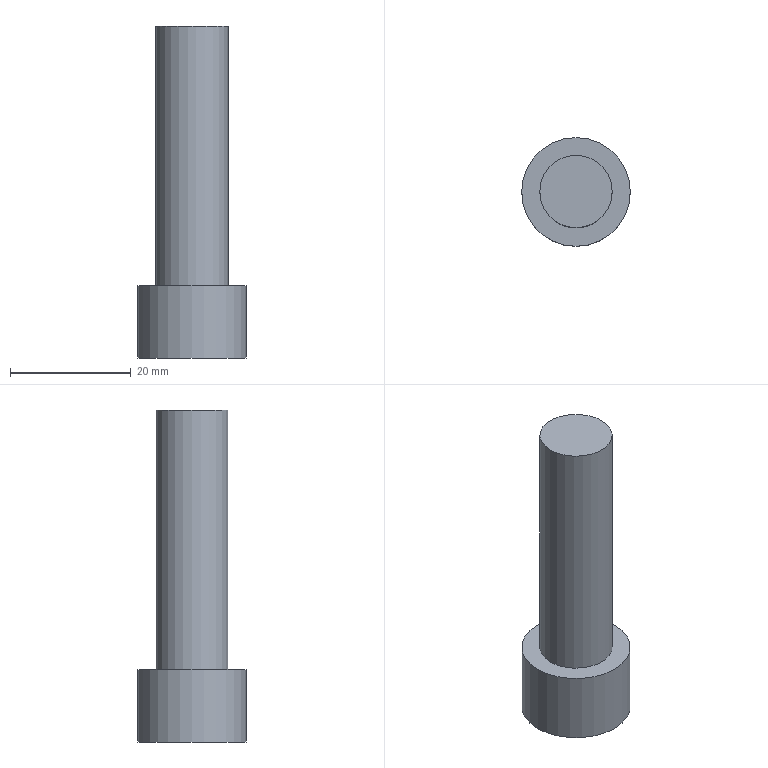Part | STEP file | 1_id610_xmt_txt | 1 solid | 18 faces | box 18 x 18 x 55 mm | volume 7362 mm3 | plane 15 | cylinder 2 | cone 1 | commonest cylinder face diameters 12 x1 18 x1
STEP:
#1=CARTESIAN_POINT('',(-111.,327.,-232.));
#2=VERTEX_POINT('',#1);
#3=CARTESIAN_POINT('',(-117.,327.,-232.));
#4=DIRECTION('',(0.,0.,-1.));
#5=DIRECTION('',(1.,0.,0.));
#6=AXIS2_PLACEMENT_3D('',#3,#4,#5);
#7=CIRCLE('',#6,6.);
#8=EDGE_CURVE('',#2,#2,#7,.T.);
#9=ORIENTED_EDGE('',*,*,#8,.F.);
#10=EDGE_LOOP('',(#9));
#11=FACE_BOUND('',#10,.T.);
#12=CARTESIAN_POINT('',(-111.,327.,-189.));
#13=VERTEX_POINT('',#12);
#14=CARTESIAN_POINT('',(-117.,327.,-189.));
#15=DIRECTION('',(0.,0.,1.));
#16=DIRECTION('',(1.,0.,0.));
#17=AXIS2_PLACEMENT_3D('',#14,#15,#16);
#18=CIRCLE('',#17,6.);
#19=EDGE_CURVE('',#13,#13,#18,.T.);
#20=ORIENTED_EDGE('',*,*,#19,.F.);
#21=EDGE_LOOP('',(#20));
#22=FACE_BOUND('',#21,.T.);
#23=CARTESIAN_POINT('',(-117.,327.,-212.));
#24=DIRECTION('',(0.,0.,1.));
#25=DIRECTION('',(-1.,0.,0.));
#26=AXIS2_PLACEMENT_3D('',#23,#24,#25);
#27=CYLINDRICAL_SURFACE('',#26,6.);
#28=ADVANCED_FACE('',(#11,#22),#27,.T.);
#29=CARTESIAN_POINT('',(-108.,327.,-244.));
#30=VERTEX_POINT('',#29);
#31=CARTESIAN_POINT('',(-117.,327.,-244.));
#32=DIRECTION('',(0.,0.,-1.));
#33=DIRECTION('',(1.,0.,0.));
#34=AXIS2_PLACEMENT_3D('',#31,#32,#33);
#35=CIRCLE('',#34,9.);
#36=EDGE_CURVE('',#30,#30,#35,.T.);
#37=ORIENTED_EDGE('',*,*,#36,.F.);
#38=EDGE_LOOP('',(#37));
#39=FACE_BOUND('',#38,.T.);
#40=CARTESIAN_POINT('',(-108.,327.,-232.));
#41=VERTEX_POINT('',#40);
#42=CARTESIAN_POINT('',(-117.,327.,-232.));
#43=DIRECTION('',(0.,0.,1.));
#44=DIRECTION('',(1.,0.,0.));
#45=AXIS2_PLACEMENT_3D('',#42,#43,#44);
#46=CIRCLE('',#45,9.);
#47=EDGE_CURVE('',#41,#41,#46,.T.);
#48=ORIENTED_EDGE('',*,*,#47,.F.);
#49=EDGE_LOOP('',(#48));
#50=FACE_BOUND('',#49,.T.);
#51=CARTESIAN_POINT('',(-117.,327.,-238.));
#52=DIRECTION('',(0.,0.,1.));
#53=DIRECTION('',(-1.,0.,0.));
#54=AXIS2_PLACEMENT_3D('',#51,#52,#53);
#55=CYLINDRICAL_SURFACE('',#54,9.);
#56=ADVANCED_FACE('',(#39,#50),#55,.T.);
#57=CARTESIAN_POINT('',(-117.,332.774,-238.));
#58=VERTEX_POINT('',#57);
#59=CARTESIAN_POINT('',(-112.,329.887,-238.));
#60=VERTEX_POINT('',#59);
#61=CARTESIAN_POINT('',(-117.,327.,-238.));
#62=DIRECTION('',(0.,0.,-1.));
#63=DIRECTION('',(1.,0.,0.));
#64=AXIS2_PLACEMENT_3D('',#61,#62,#63);
#65=CIRCLE('',#64,5.774);
#66=EDGE_CURVE('',#58,#60,#65,.T.);
#67=ORIENTED_EDGE('',*,*,#66,.T.);
#68=CARTESIAN_POINT('',(-112.,324.113,-238.));
#69=VERTEX_POINT('',#68);
#70=CARTESIAN_POINT('',(-117.,327.,-238.));
#71=DIRECTION('',(0.,0.,-1.));
#72=DIRECTION('',(1.,0.,0.));
#73=AXIS2_PLACEMENT_3D('',#70,#71,#72);
#74=CIRCLE('',#73,5.774);
#75=EDGE_CURVE('',#60,#69,#74,.T.);
#76=ORIENTED_EDGE('',*,*,#75,.T.);
#77=CARTESIAN_POINT('',(-117.,321.226,-238.));
#78=VERTEX_POINT('',#77);
#79=CARTESIAN_POINT('',(-117.,327.,-238.));
#80=DIRECTION('',(0.,0.,-1.));
#81=DIRECTION('',(1.,0.,0.));
#82=AXIS2_PLACEMENT_3D('',#79,#80,#81);
#83=CIRCLE('',#82,5.774);
#84=EDGE_CURVE('',#69,#78,#83,.T.);
#85=ORIENTED_EDGE('',*,*,#84,.T.);
#86=CARTESIAN_POINT('',(-122.,324.113,-238.));
#87=VERTEX_POINT('',#86);
#88=CARTESIAN_POINT('',(-117.,327.,-238.));
#89=DIRECTION('',(0.,0.,-1.));
#90=DIRECTION('',(1.,0.,0.));
#91=AXIS2_PLACEMENT_3D('',#88,#89,#90);
#92=CIRCLE('',#91,5.774);
#93=EDGE_CURVE('',#78,#87,#92,.T.);
#94=ORIENTED_EDGE('',*,*,#93,.T.);
#95=CARTESIAN_POINT('',(-122.,329.887,-238.));
#96=VERTEX_POINT('',#95);
#97=CARTESIAN_POINT('',(-117.,327.,-238.));
#98=DIRECTION('',(0.,0.,-1.));
#99=DIRECTION('',(1.,0.,0.));
#100=AXIS2_PLACEMENT_3D('',#97,#98,#99);
#101=CIRCLE('',#100,5.774);
#102=EDGE_CURVE('',#87,#96,#101,.T.);
#103=ORIENTED_EDGE('',*,*,#102,.T.);
#104=CARTESIAN_POINT('',(-117.,327.,-238.));
#105=DIRECTION('',(0.,0.,-1.));
#106=DIRECTION('',(1.,0.,0.));
#107=AXIS2_PLACEMENT_3D('',#104,#105,#106);
#108=CIRCLE('',#107,5.774);
#109=EDGE_CURVE('',#96,#58,#108,.T.);
#110=ORIENTED_EDGE('',*,*,#109,.T.);
#111=EDGE_LOOP('',(#67,#76,#85,#94,#103,#110));
#112=FACE_BOUND('',#111,.T.);
#113=CARTESIAN_POINT('',(-117.,327.,-237.));
#114=VERTEX_POINT('',#113);
#115=VERTEX_LOOP('',#114);
#116=FACE_BOUND('',#115,.T.);
#117=CARTESIAN_POINT('',(-117.,327.,-237.5));
#118=DIRECTION('',(0.,0.,-1.));
#119=DIRECTION('',(-1.,0.,0.));
#120=AXIS2_PLACEMENT_3D('',#117,#118,#119);
#121=CONICAL_SURFACE('',#120,2.887,80.174);
#122=ADVANCED_FACE('',(#112,#116),#121,.F.);
#123=CARTESIAN_POINT('',(-114.5,322.67,-238.));
#124=DIRECTION('',(0.866,0.5,0.));
#125=VECTOR('',#124,1.);
#126=LINE('',#123,#125);
#127=EDGE_CURVE('',#78,#69,#126,.T.);
#128=ORIENTED_EDGE('',*,*,#127,.F.);
#129=ORIENTED_EDGE('',*,*,#84,.F.);
#130=EDGE_LOOP('',(#128,#129));
#131=FACE_OUTER_BOUND('',#130,.T.);
#132=CARTESIAN_POINT('',(-117.,327.,-238.));
#133=DIRECTION('',(0.,0.,-1.));
#134=DIRECTION('',(1.,0.,0.));
#135=AXIS2_PLACEMENT_3D('',#132,#133,#134);
#136=PLANE('',#135);
#137=ADVANCED_FACE('',(#131),#136,.F.);
#138=CARTESIAN_POINT('',(-112.,327.,-238.));
#139=DIRECTION('',(0.,1.,0.));
#140=VECTOR('',#139,1.);
#141=LINE('',#138,#140);
#142=EDGE_CURVE('',#69,#60,#141,.T.);
#143=ORIENTED_EDGE('',*,*,#142,.F.);
#144=ORIENTED_EDGE('',*,*,#75,.F.);
#145=EDGE_LOOP('',(#143,#144));
#146=FACE_OUTER_BOUND('',#145,.T.);
#147=CARTESIAN_POINT('',(-117.,327.,-238.));
#148=DIRECTION('',(0.,0.,-1.));
#149=DIRECTION('',(1.,0.,0.));
#150=AXIS2_PLACEMENT_3D('',#147,#148,#149);
#151=PLANE('',#150);
#152=ADVANCED_FACE('',(#146),#151,.F.);
#153=CARTESIAN_POINT('',(-114.5,331.33,-238.));
#154=DIRECTION('',(-0.866,0.5,0.));
#155=VECTOR('',#154,1.);
#156=LINE('',#153,#155);
#157=EDGE_CURVE('',#60,#58,#156,.T.);
#158=ORIENTED_EDGE('',*,*,#157,.F.);
#159=ORIENTED_EDGE('',*,*,#66,.F.);
#160=EDGE_LOOP('',(#158,#159));
#161=FACE_OUTER_BOUND('',#160,.T.);
#162=CARTESIAN_POINT('',(-117.,327.,-238.));
#163=DIRECTION('',(0.,0.,-1.));
#164=DIRECTION('',(1.,0.,0.));
#165=AXIS2_PLACEMENT_3D('',#162,#163,#164);
#166=PLANE('',#165);
#167=ADVANCED_FACE('',(#161),#166,.F.);
#168=CARTESIAN_POINT('',(-119.5,331.33,-238.));
#169=DIRECTION('',(-0.866,-0.5,0.));
#170=VECTOR('',#169,1.);
#171=LINE('',#168,#170);
#172=EDGE_CURVE('',#58,#96,#171,.T.);
#173=ORIENTED_EDGE('',*,*,#172,.F.);
#174=ORIENTED_EDGE('',*,*,#109,.F.);
#175=EDGE_LOOP('',(#173,#174));
#176=FACE_OUTER_BOUND('',#175,.T.);
#177=CARTESIAN_POINT('',(-117.,327.,-238.));
#178=DIRECTION('',(0.,0.,-1.));
#179=DIRECTION('',(1.,0.,0.));
#180=AXIS2_PLACEMENT_3D('',#177,#178,#179);
#181=PLANE('',#180);
#182=ADVANCED_FACE('',(#176),#181,.F.);
#183=CARTESIAN_POINT('',(-122.,327.,-238.));
#184=DIRECTION('',(0.,-1.,0.));
#185=VECTOR('',#184,1.);
#186=LINE('',#183,#185);
#187=EDGE_CURVE('',#96,#87,#186,.T.);
#188=ORIENTED_EDGE('',*,*,#187,.F.);
#189=ORIENTED_EDGE('',*,*,#102,.F.);
#190=EDGE_LOOP('',(#188,#189));
#191=FACE_OUTER_BOUND('',#190,.T.);
#192=CARTESIAN_POINT('',(-117.,327.,-238.));
#193=DIRECTION('',(0.,0.,-1.));
#194=DIRECTION('',(1.,0.,0.));
#195=AXIS2_PLACEMENT_3D('',#192,#193,#194);
#196=PLANE('',#195);
#197=ADVANCED_FACE('',(#191),#196,.F.);
#198=CARTESIAN_POINT('',(-119.5,322.67,-238.));
#199=DIRECTION('',(0.866,-0.5,0.));
#200=VECTOR('',#199,1.);
#201=LINE('',#198,#200);
#202=EDGE_CURVE('',#87,#78,#201,.T.);
#203=ORIENTED_EDGE('',*,*,#202,.F.);
#204=ORIENTED_EDGE('',*,*,#93,.F.);
#205=EDGE_LOOP('',(#203,#204));
#206=FACE_OUTER_BOUND('',#205,.T.);
#207=CARTESIAN_POINT('',(-117.,327.,-238.));
#208=DIRECTION('',(0.,0.,-1.));
#209=DIRECTION('',(1.,0.,0.));
#210=AXIS2_PLACEMENT_3D('',#207,#208,#209);
#211=PLANE('',#210);
#212=ADVANCED_FACE('',(#206),#211,.F.);
#213=CARTESIAN_POINT('',(-117.,321.226,-244.));
#214=VERTEX_POINT('',#213);
#215=CARTESIAN_POINT('',(-117.,321.226,-241.));
#216=DIRECTION('',(0.,0.,-1.));
#217=VECTOR('',#216,1.);
#218=LINE('',#215,#217);
#219=EDGE_CURVE('',#78,#214,#218,.T.);
#220=ORIENTED_EDGE('',*,*,#219,.F.);
#221=ORIENTED_EDGE('',*,*,#127,.T.);
#222=CARTESIAN_POINT('',(-112.,324.113,-244.));
#223=VERTEX_POINT('',#222);
#224=CARTESIAN_POINT('',(-112.,324.113,-241.));
#225=DIRECTION('',(0.,0.,-1.));
#226=VECTOR('',#225,1.);
#227=LINE('',#224,#226);
#228=EDGE_CURVE('',#69,#223,#227,.T.);
#229=ORIENTED_EDGE('',*,*,#228,.T.);
#230=CARTESIAN_POINT('',(-114.5,322.67,-244.));
#231=DIRECTION('',(0.866,0.5,0.));
#232=VECTOR('',#231,1.);
#233=LINE('',#230,#232);
#234=EDGE_CURVE('',#214,#223,#233,.T.);
#235=ORIENTED_EDGE('',*,*,#234,.F.);
#236=EDGE_LOOP('',(#220,#221,#229,#235));
#237=FACE_OUTER_BOUND('',#236,.T.);
#238=CARTESIAN_POINT('',(-114.5,322.67,-241.));
#239=DIRECTION('',(-0.5,0.866,0.));
#240=DIRECTION('',(0.,0.,-1.));
#241=AXIS2_PLACEMENT_3D('',#238,#239,#240);
#242=PLANE('',#241);
#243=ADVANCED_FACE('',(#237),#242,.T.);
#244=CARTESIAN_POINT('',(-122.,324.113,-244.));
#245=VERTEX_POINT('',#244);
#246=CARTESIAN_POINT('',(-122.,324.113,-241.));
#247=DIRECTION('',(0.,0.,-1.));
#248=VECTOR('',#247,1.);
#249=LINE('',#246,#248);
#250=EDGE_CURVE('',#87,#245,#249,.T.);
#251=ORIENTED_EDGE('',*,*,#250,.F.);
#252=ORIENTED_EDGE('',*,*,#202,.T.);
#253=ORIENTED_EDGE('',*,*,#219,.T.);
#254=CARTESIAN_POINT('',(-119.5,322.67,-244.));
#255=DIRECTION('',(0.866,-0.5,0.));
#256=VECTOR('',#255,1.);
#257=LINE('',#254,#256);
#258=EDGE_CURVE('',#245,#214,#257,.T.);
#259=ORIENTED_EDGE('',*,*,#258,.F.);
#260=EDGE_LOOP('',(#251,#252,#253,#259));
#261=FACE_OUTER_BOUND('',#260,.T.);
#262=CARTESIAN_POINT('',(-119.5,322.67,-241.));
#263=DIRECTION('',(0.5,0.866,0.));
#264=DIRECTION('',(0.,0.,1.));
#265=AXIS2_PLACEMENT_3D('',#262,#263,#264);
#266=PLANE('',#265);
#267=ADVANCED_FACE('',(#261),#266,.T.);
#268=CARTESIAN_POINT('',(-122.,329.887,-244.));
#269=VERTEX_POINT('',#268);
#270=CARTESIAN_POINT('',(-122.,329.887,-241.));
#271=DIRECTION('',(0.,0.,-1.));
#272=VECTOR('',#271,1.);
#273=LINE('',#270,#272);
#274=EDGE_CURVE('',#96,#269,#273,.T.);
#275=ORIENTED_EDGE('',*,*,#274,.F.);
#276=ORIENTED_EDGE('',*,*,#187,.T.);
#277=ORIENTED_EDGE('',*,*,#250,.T.);
#278=CARTESIAN_POINT('',(-122.,327.,-244.));
#279=DIRECTION('',(0.,-1.,0.));
#280=VECTOR('',#279,1.);
#281=LINE('',#278,#280);
#282=EDGE_CURVE('',#269,#245,#281,.T.);
#283=ORIENTED_EDGE('',*,*,#282,.F.);
#284=EDGE_LOOP('',(#275,#276,#277,#283));
#285=FACE_OUTER_BOUND('',#284,.T.);
#286=CARTESIAN_POINT('',(-122.,327.,-241.));
#287=DIRECTION('',(1.,0.,0.));
#288=DIRECTION('',(0.,0.,1.));
#289=AXIS2_PLACEMENT_3D('',#286,#287,#288);
#290=PLANE('',#289);
#291=ADVANCED_FACE('',(#285),#290,.T.);
#292=CARTESIAN_POINT('',(-117.,332.774,-244.));
#293=VERTEX_POINT('',#292);
#294=CARTESIAN_POINT('',(-117.,332.774,-241.));
#295=DIRECTION('',(0.,0.,-1.));
#296=VECTOR('',#295,1.);
#297=LINE('',#294,#296);
#298=EDGE_CURVE('',#58,#293,#297,.T.);
#299=ORIENTED_EDGE('',*,*,#298,.F.);
#300=ORIENTED_EDGE('',*,*,#172,.T.);
#301=ORIENTED_EDGE('',*,*,#274,.T.);
#302=CARTESIAN_POINT('',(-119.5,331.33,-244.));
#303=DIRECTION('',(-0.866,-0.5,0.));
#304=VECTOR('',#303,1.);
#305=LINE('',#302,#304);
#306=EDGE_CURVE('',#293,#269,#305,.T.);
#307=ORIENTED_EDGE('',*,*,#306,.F.);
#308=EDGE_LOOP('',(#299,#300,#301,#307));
#309=FACE_OUTER_BOUND('',#308,.T.);
#310=CARTESIAN_POINT('',(-119.5,331.33,-241.));
#311=DIRECTION('',(0.5,-0.866,0.));
#312=DIRECTION('',(0.,0.,1.));
#313=AXIS2_PLACEMENT_3D('',#310,#311,#312);
#314=PLANE('',#313);
#315=ADVANCED_FACE('',(#309),#314,.T.);
#316=CARTESIAN_POINT('',(-112.,329.887,-244.));
#317=VERTEX_POINT('',#316);
#318=CARTESIAN_POINT('',(-112.,329.887,-241.));
#319=DIRECTION('',(0.,0.,-1.));
#320=VECTOR('',#319,1.);
#321=LINE('',#318,#320);
#322=EDGE_CURVE('',#60,#317,#321,.T.);
#323=ORIENTED_EDGE('',*,*,#322,.F.);
#324=ORIENTED_EDGE('',*,*,#157,.T.);
#325=ORIENTED_EDGE('',*,*,#298,.T.);
#326=CARTESIAN_POINT('',(-114.5,331.33,-244.));
#327=DIRECTION('',(-0.866,0.5,0.));
#328=VECTOR('',#327,1.);
#329=LINE('',#326,#328);
#330=EDGE_CURVE('',#317,#293,#329,.T.);
#331=ORIENTED_EDGE('',*,*,#330,.F.);
#332=EDGE_LOOP('',(#323,#324,#325,#331));
#333=FACE_OUTER_BOUND('',#332,.T.);
#334=CARTESIAN_POINT('',(-114.5,331.33,-241.));
#335=DIRECTION('',(-0.5,-0.866,0.));
#336=DIRECTION('',(0.,0.,-1.));
#337=AXIS2_PLACEMENT_3D('',#334,#335,#336);
#338=PLANE('',#337);
#339=ADVANCED_FACE('',(#333),#338,.T.);
#340=ORIENTED_EDGE('',*,*,#228,.F.);
#341=ORIENTED_EDGE('',*,*,#142,.T.);
#342=ORIENTED_EDGE('',*,*,#322,.T.);
#343=CARTESIAN_POINT('',(-112.,327.,-244.));
#344=DIRECTION('',(0.,1.,0.));
#345=VECTOR('',#344,1.);
#346=LINE('',#343,#345);
#347=EDGE_CURVE('',#223,#317,#346,.T.);
#348=ORIENTED_EDGE('',*,*,#347,.F.);
#349=EDGE_LOOP('',(#340,#341,#342,#348));
#350=FACE_OUTER_BOUND('',#349,.T.);
#351=CARTESIAN_POINT('',(-112.,327.,-241.));
#352=DIRECTION('',(-1.,0.,0.));
#353=DIRECTION('',(0.,0.,-1.));
#354=AXIS2_PLACEMENT_3D('',#351,#352,#353);
#355=PLANE('',#354);
#356=ADVANCED_FACE('',(#350),#355,.T.);
#357=ORIENTED_EDGE('',*,*,#234,.T.);
#358=ORIENTED_EDGE('',*,*,#347,.T.);
#359=ORIENTED_EDGE('',*,*,#330,.T.);
#360=ORIENTED_EDGE('',*,*,#306,.T.);
#361=ORIENTED_EDGE('',*,*,#282,.T.);
#362=ORIENTED_EDGE('',*,*,#258,.T.);
#363=EDGE_LOOP('',(#357,#358,#359,#360,#361,#362));
#364=FACE_BOUND('',#363,.T.);
#365=ORIENTED_EDGE('',*,*,#36,.T.);
#366=EDGE_LOOP('',(#365));
#367=FACE_BOUND('',#366,.T.);
#368=CARTESIAN_POINT('',(-117.,327.,-244.));
#369=DIRECTION('',(0.,0.,-1.));
#370=DIRECTION('',(1.,0.,0.));
#371=AXIS2_PLACEMENT_3D('',#368,#369,#370);
#372=PLANE('',#371);
#373=ADVANCED_FACE('',(#364,#367),#372,.T.);
#374=ORIENTED_EDGE('',*,*,#8,.T.);
#375=EDGE_LOOP('',(#374));
#376=FACE_BOUND('',#375,.T.);
#377=ORIENTED_EDGE('',*,*,#47,.T.);
#378=EDGE_LOOP('',(#377));
#379=FACE_BOUND('',#378,.T.);
#380=CARTESIAN_POINT('',(-117.,327.,-232.));
#381=DIRECTION('',(0.,0.,1.));
#382=DIRECTION('',(-1.,0.,0.));
#383=AXIS2_PLACEMENT_3D('',#380,#381,#382);
#384=PLANE('',#383);
#385=ADVANCED_FACE('',(#376,#379),#384,.T.);
#386=ORIENTED_EDGE('',*,*,#19,.T.);
#387=EDGE_LOOP('',(#386));
#388=FACE_OUTER_BOUND('',#387,.T.);
#389=CARTESIAN_POINT('',(0.,90.,-189.));
#390=DIRECTION('',(0.,0.,1.));
#391=DIRECTION('',(1.,0.,0.));
#392=AXIS2_PLACEMENT_3D('',#389,#390,#391);
#393=PLANE('',#392);
#394=ADVANCED_FACE('',(#388),#393,.T.);
#395=CLOSED_SHELL('',(#28,#56,#122,#137,#152,#167,#182,#197,#212,#243,#267,#291,#315,#339,#356,#373,#385,#394));
#396=MANIFOLD_SOLID_BREP('',#395);
#397=(LENGTH_UNIT()NAMED_UNIT(*)SI_UNIT(.MILLI.,.METRE.));
#398=UNCERTAINTY_MEASURE_WITH_UNIT(LENGTH_MEASURE(0.00002),#397,'','');
#399=(NAMED_UNIT(*)PLANE_ANGLE_UNIT()SI_UNIT($,.RADIAN.));
#400=PLANE_ANGLE_MEASURE_WITH_UNIT(PLANE_ANGLE_MEASURE(0.01745),#399);
#401=DIMENSIONAL_EXPONENTS(0.,0.,0.,0.,0.,0.,0.);
#402=(CONVERSION_BASED_UNIT('DEGREE',#400)NAMED_UNIT(#401)PLANE_ANGLE_UNIT());
#403=(NAMED_UNIT(*)SI_UNIT($,.STERADIAN.)SOLID_ANGLE_UNIT());
#404=(GEOMETRIC_REPRESENTATION_CONTEXT(3)GLOBAL_UNCERTAINTY_ASSIGNED_CONTEXT((#398))GLOBAL_UNIT_ASSIGNED_CONTEXT((#397,#402,#403))REPRESENTATION_CONTEXT('',''));
#405=ADVANCED_BREP_SHAPE_REPRESENTATION('',(#396),#404);